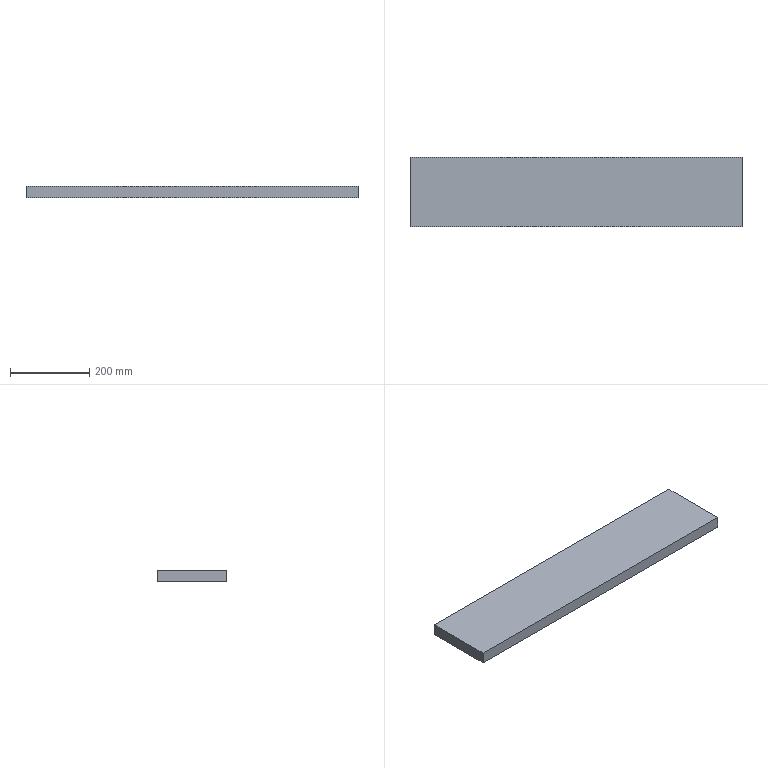Part | SolidWorks | features Extrusion 1 | 1 solid | 6 faces | box 840 x 175 x 30 mm | volume 4410000 mm3 | plane 6
STEP:
#1=CARTESIAN_POINT('',(0.,175.,0.));
#2=VERTEX_POINT('',#1);
#3=CARTESIAN_POINT('',(0.,0.,0.));
#4=VERTEX_POINT('',#3);
#5=CARTESIAN_POINT('',(0.,0.,0.));
#6=DIRECTION('',(0.,-1.,0.));
#7=VECTOR('',#6,1000.);
#8=LINE('',#5,#7);
#9=EDGE_CURVE('',#2,#4,#8,.T.);
#10=ORIENTED_EDGE('',*,*,#9,.T.);
#11=CARTESIAN_POINT('',(0.,0.,30.));
#12=VERTEX_POINT('',#11);
#13=CARTESIAN_POINT('',(0.,0.,30.));
#14=DIRECTION('',(0.,0.,-1.));
#15=VECTOR('',#14,1000.);
#16=LINE('',#13,#15);
#17=EDGE_CURVE('',#12,#4,#16,.T.);
#18=ORIENTED_EDGE('',*,*,#17,.F.);
#19=CARTESIAN_POINT('',(0.,175.,30.));
#20=VERTEX_POINT('',#19);
#21=CARTESIAN_POINT('',(0.,0.,30.));
#22=DIRECTION('',(0.,-1.,0.));
#23=VECTOR('',#22,1000.);
#24=LINE('',#21,#23);
#25=EDGE_CURVE('',#20,#12,#24,.T.);
#26=ORIENTED_EDGE('',*,*,#25,.F.);
#27=CARTESIAN_POINT('',(0.,175.,30.));
#28=DIRECTION('',(0.,0.,-1.));
#29=VECTOR('',#28,1000.);
#30=LINE('',#27,#29);
#31=EDGE_CURVE('',#20,#2,#30,.T.);
#32=ORIENTED_EDGE('',*,*,#31,.T.);
#33=EDGE_LOOP('',(#10,#18,#26,#32));
#34=FACE_OUTER_BOUND('',#33,.T.);
#35=CARTESIAN_POINT('',(0.,0.,30.));
#36=DIRECTION('',(1.,0.,0.));
#37=DIRECTION('',(0.,0.,-1.));
#38=AXIS2_PLACEMENT_3D('',#35,#36,#37);
#39=PLANE('',#38);
#40=ADVANCED_FACE('',(#34),#39,.F.);
#41=CARTESIAN_POINT('',(840.,0.,0.));
#42=VERTEX_POINT('',#41);
#43=CARTESIAN_POINT('',(0.,0.,0.));
#44=DIRECTION('',(1.,0.,0.));
#45=VECTOR('',#44,1000.);
#46=LINE('',#43,#45);
#47=EDGE_CURVE('',#4,#42,#46,.T.);
#48=ORIENTED_EDGE('',*,*,#47,.T.);
#49=CARTESIAN_POINT('',(840.,0.,30.));
#50=VERTEX_POINT('',#49);
#51=CARTESIAN_POINT('',(840.,0.,30.));
#52=DIRECTION('',(0.,0.,-1.));
#53=VECTOR('',#52,1000.);
#54=LINE('',#51,#53);
#55=EDGE_CURVE('',#50,#42,#54,.T.);
#56=ORIENTED_EDGE('',*,*,#55,.F.);
#57=CARTESIAN_POINT('',(0.,0.,30.));
#58=DIRECTION('',(1.,0.,0.));
#59=VECTOR('',#58,1000.);
#60=LINE('',#57,#59);
#61=EDGE_CURVE('',#12,#50,#60,.T.);
#62=ORIENTED_EDGE('',*,*,#61,.F.);
#63=ORIENTED_EDGE('',*,*,#17,.T.);
#64=EDGE_LOOP('',(#48,#56,#62,#63));
#65=FACE_OUTER_BOUND('',#64,.T.);
#66=CARTESIAN_POINT('',(0.,0.,30.));
#67=DIRECTION('',(0.,1.,0.));
#68=DIRECTION('',(0.,0.,1.));
#69=AXIS2_PLACEMENT_3D('',#66,#67,#68);
#70=PLANE('',#69);
#71=ADVANCED_FACE('',(#65),#70,.F.);
#72=CARTESIAN_POINT('',(840.,175.,0.));
#73=VERTEX_POINT('',#72);
#74=CARTESIAN_POINT('',(840.,0.,0.));
#75=DIRECTION('',(0.,1.,0.));
#76=VECTOR('',#75,1000.);
#77=LINE('',#74,#76);
#78=EDGE_CURVE('',#42,#73,#77,.T.);
#79=ORIENTED_EDGE('',*,*,#78,.T.);
#80=CARTESIAN_POINT('',(840.,175.,30.));
#81=VERTEX_POINT('',#80);
#82=CARTESIAN_POINT('',(840.,175.,30.));
#83=DIRECTION('',(0.,0.,-1.));
#84=VECTOR('',#83,1000.);
#85=LINE('',#82,#84);
#86=EDGE_CURVE('',#81,#73,#85,.T.);
#87=ORIENTED_EDGE('',*,*,#86,.F.);
#88=CARTESIAN_POINT('',(840.,0.,30.));
#89=DIRECTION('',(0.,1.,0.));
#90=VECTOR('',#89,1000.);
#91=LINE('',#88,#90);
#92=EDGE_CURVE('',#50,#81,#91,.T.);
#93=ORIENTED_EDGE('',*,*,#92,.F.);
#94=ORIENTED_EDGE('',*,*,#55,.T.);
#95=EDGE_LOOP('',(#79,#87,#93,#94));
#96=FACE_OUTER_BOUND('',#95,.T.);
#97=CARTESIAN_POINT('',(840.,0.,30.));
#98=DIRECTION('',(-1.,0.,0.));
#99=DIRECTION('',(0.,0.,1.));
#100=AXIS2_PLACEMENT_3D('',#97,#98,#99);
#101=PLANE('',#100);
#102=ADVANCED_FACE('',(#96),#101,.F.);
#103=CARTESIAN_POINT('',(0.,175.,0.));
#104=DIRECTION('',(-1.,0.,0.));
#105=VECTOR('',#104,1000.);
#106=LINE('',#103,#105);
#107=EDGE_CURVE('',#73,#2,#106,.T.);
#108=ORIENTED_EDGE('',*,*,#107,.T.);
#109=ORIENTED_EDGE('',*,*,#31,.F.);
#110=CARTESIAN_POINT('',(0.,175.,30.));
#111=DIRECTION('',(-1.,0.,0.));
#112=VECTOR('',#111,1000.);
#113=LINE('',#110,#112);
#114=EDGE_CURVE('',#81,#20,#113,.T.);
#115=ORIENTED_EDGE('',*,*,#114,.F.);
#116=ORIENTED_EDGE('',*,*,#86,.T.);
#117=EDGE_LOOP('',(#108,#109,#115,#116));
#118=FACE_OUTER_BOUND('',#117,.T.);
#119=CARTESIAN_POINT('',(0.,175.,30.));
#120=DIRECTION('',(0.,-1.,0.));
#121=DIRECTION('',(1.,0.,0.));
#122=AXIS2_PLACEMENT_3D('',#119,#120,#121);
#123=PLANE('',#122);
#124=ADVANCED_FACE('',(#118),#123,.F.);
#125=ORIENTED_EDGE('',*,*,#25,.T.);
#126=ORIENTED_EDGE('',*,*,#61,.T.);
#127=ORIENTED_EDGE('',*,*,#92,.T.);
#128=ORIENTED_EDGE('',*,*,#114,.T.);
#129=EDGE_LOOP('',(#125,#126,#127,#128));
#130=FACE_OUTER_BOUND('',#129,.T.);
#131=CARTESIAN_POINT('',(0.,0.,30.));
#132=DIRECTION('',(0.,0.,-1.));
#133=DIRECTION('',(-1.,0.,0.));
#134=AXIS2_PLACEMENT_3D('',#131,#132,#133);
#135=PLANE('',#134);
#136=ADVANCED_FACE('',(#130),#135,.F.);
#137=ORIENTED_EDGE('',*,*,#9,.F.);
#138=ORIENTED_EDGE('',*,*,#107,.F.);
#139=ORIENTED_EDGE('',*,*,#78,.F.);
#140=ORIENTED_EDGE('',*,*,#47,.F.);
#141=EDGE_LOOP('',(#137,#138,#139,#140));
#142=FACE_OUTER_BOUND('',#141,.T.);
#143=CARTESIAN_POINT('',(0.,0.,0.));
#144=DIRECTION('',(0.,0.,-1.));
#145=DIRECTION('',(-1.,0.,0.));
#146=AXIS2_PLACEMENT_3D('',#143,#144,#145);
#147=PLANE('',#146);
#148=ADVANCED_FACE('',(#142),#147,.T.);
#149=CLOSED_SHELL('',(#40,#71,#102,#124,#136,#148));
#150=MANIFOLD_SOLID_BREP('',#149);
#151=CARTESIAN_POINT('',(0.,0.,0.));
#152=DIRECTION('',(0.,0.,1.));
#153=DIRECTION('',(1.,0.,0.));
#154=AXIS2_PLACEMENT_3D('',#151,#152,#153);
#155=(LENGTH_UNIT()NAMED_UNIT(*)SI_UNIT(.MILLI.,.METRE.));
#156=UNCERTAINTY_MEASURE_WITH_UNIT(LENGTH_MEASURE(0.00001),#155,'','');
#157=(NAMED_UNIT(*)PLANE_ANGLE_UNIT()SI_UNIT($,.RADIAN.));
#158=(NAMED_UNIT(*)SI_UNIT($,.STERADIAN.)SOLID_ANGLE_UNIT());
#159=(GEOMETRIC_REPRESENTATION_CONTEXT(3)GLOBAL_UNCERTAINTY_ASSIGNED_CONTEXT((#156))GLOBAL_UNIT_ASSIGNED_CONTEXT((#155,#157,#158))REPRESENTATION_CONTEXT('',''));
#160=ADVANCED_BREP_SHAPE_REPRESENTATION('',(#150,#154),#159);